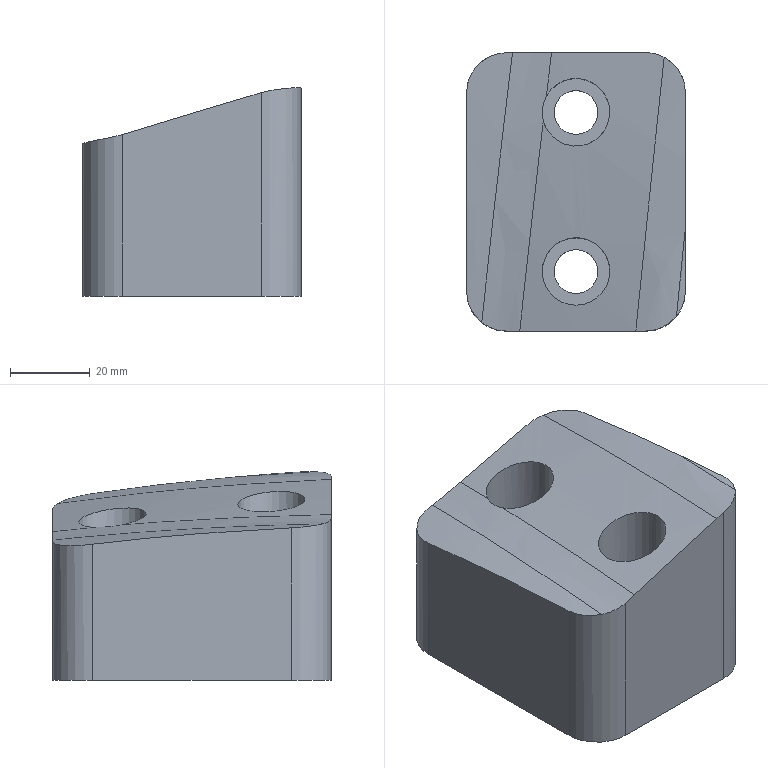Part | NX | features solid 2 | 1 solid | 20 faces | box 55 x 70 x 52.401 mm | volume 147496 mm3 | cylinder 8 | plane 7 | spline 5 | commonest cylinder face diameters 20 x4 11 x2 17 x2
STEP:
#1=CARTESIAN_POINT('',(-250.,310.,23.05));
#2=VERTEX_POINT('',#1);
#3=CARTESIAN_POINT('',(-273.631,310.,17.313));
#4=VERTEX_POINT('',#3);
#5=CARTESIAN_POINT('',(-250.,310.,23.05));
#6=CARTESIAN_POINT('',(-257.879,310.,21.145));
#7=CARTESIAN_POINT('',(-265.756,310.,19.234));
#8=CARTESIAN_POINT('',(-273.631,310.,17.313));
#9=B_SPLINE_CURVE_WITH_KNOTS('',3,(#5,#6,#7,#8),.UNSPECIFIED.,.F.,.F.,(4,4),(0.005181,0.0295),.UNSPECIFIED.);
#10=EDGE_CURVE('',#2,#4,#9,.T.);
#11=ORIENTED_EDGE('',*,*,#10,.T.);
#12=CARTESIAN_POINT('',(-274.974,299.048,18.446));
#13=VERTEX_POINT('',#12);
#14=CARTESIAN_POINT('',(-273.631,310.,17.313));
#15=CARTESIAN_POINT('',(-274.07,306.431,17.719));
#16=CARTESIAN_POINT('',(-274.514,302.785,18.097));
#17=CARTESIAN_POINT('',(-274.965,299.055,18.448));
#18=B_SPLINE_CURVE_WITH_KNOTS('',3,(#14,#15,#16,#17),.UNSPECIFIED.,.F.,.F.,(4,4),(0.03901,0.4464),.UNSPECIFIED.);
#19=EDGE_CURVE('',#4,#13,#18,.T.);
#20=ORIENTED_EDGE('',*,*,#19,.T.);
#21=CARTESIAN_POINT('',(-275.72,292.836,18.999));
#22=VERTEX_POINT('',#21);
#23=CARTESIAN_POINT('',(-274.963,299.068,18.447));
#24=CARTESIAN_POINT('',(-274.01,300.817,18.471));
#25=CARTESIAN_POINT('',(-270.799,303.603,18.912));
#26=CARTESIAN_POINT('',(-264.634,303.713,20.424));
#27=CARTESIAN_POINT('',(-259.81,300.02,22.155));
#28=CARTESIAN_POINT('',(-258.326,293.943,23.371));
#29=CARTESIAN_POINT('',(-261.238,288.212,23.347));
#30=CARTESIAN_POINT('',(-267.031,285.826,22.093));
#31=CARTESIAN_POINT('',(-272.858,287.562,20.346));
#32=CARTESIAN_POINT('',(-275.205,290.9,19.356));
#33=CARTESIAN_POINT('',(-275.715,292.816,19.003));
#34=B_SPLINE_CURVE_WITH_KNOTS('',3,(#23,#24,#25,#26,#27,#28,#29,#30,#31,#32,#33),.UNSPECIFIED.,.F.,.F.,(4,1,1,1,1,1,1,1,4),(0.001597,0.007571,0.01355,0.01952,0.02549,0.03147,0.03744,0.04341,0.04939),.UNSPECIFIED.);
#35=EDGE_CURVE('',#13,#22,#34,.T.);
#36=ORIENTED_EDGE('',*,*,#35,.T.);
#37=CARTESIAN_POINT('',(-276.835,283.374,19.727));
#38=VERTEX_POINT('',#37);
#39=CARTESIAN_POINT('',(-275.713,292.829,19.002));
#40=CARTESIAN_POINT('',(-276.083,289.735,19.261));
#41=CARTESIAN_POINT('',(-276.457,286.584,19.503));
#42=CARTESIAN_POINT('',(-276.835,283.374,19.727));
#43=B_SPLINE_CURVE_WITH_KNOTS('',3,(#39,#40,#41,#42),.UNSPECIFIED.,.F.,.F.,(4,4),(0.6703,1.),.UNSPECIFIED.);
#44=EDGE_CURVE('',#22,#38,#43,.T.);
#45=ORIENTED_EDGE('',*,*,#44,.T.);
#46=CARTESIAN_POINT('',(-281.649,240.,21.629));
#47=VERTEX_POINT('',#46);
#48=CARTESIAN_POINT('',(-276.835,283.374,19.727));
#49=CARTESIAN_POINT('',(-278.37,270.039,20.667));
#50=CARTESIAN_POINT('',(-279.977,255.669,21.299));
#51=CARTESIAN_POINT('',(-281.671,240.002,21.622));
#52=B_SPLINE_CURVE_WITH_KNOTS('',3,(#48,#49,#50,#51),.UNSPECIFIED.,.F.,.F.,(4,4),(0.,1.502),.UNSPECIFIED.);
#53=EDGE_CURVE('',#38,#47,#52,.T.);
#54=ORIENTED_EDGE('',*,*,#53,.T.);
#55=CARTESIAN_POINT('',(-252.459,240.,30.481));
#56=VERTEX_POINT('',#55);
#57=CARTESIAN_POINT('',(-252.459,240.,30.481));
#58=CARTESIAN_POINT('',(-262.204,240.,27.579));
#59=CARTESIAN_POINT('',(-271.934,240.,24.63));
#60=CARTESIAN_POINT('',(-281.649,240.,21.629));
#61=B_SPLINE_CURVE_WITH_KNOTS('',3,(#57,#58,#59,#60),.UNSPECIFIED.,.F.,.F.,(4,4),(0.1228,0.1533),.UNSPECIFIED.);
#62=EDGE_CURVE('',#47,#56,#61,.F.);
#63=ORIENTED_EDGE('',*,*,#62,.T.);
#64=CARTESIAN_POINT('',(-247.544,288.029,26.924));
#65=VERTEX_POINT('',#64);
#66=CARTESIAN_POINT('',(-252.459,240.,30.481));
#67=CARTESIAN_POINT('',(-250.751,256.963,29.719));
#68=CARTESIAN_POINT('',(-249.117,272.921,28.534));
#69=CARTESIAN_POINT('',(-247.544,288.029,26.924));
#70=B_SPLINE_CURVE_WITH_KNOTS('',3,(#66,#67,#68,#69),.UNSPECIFIED.,.F.,.F.,(4,4),(0.02255,1.),.UNSPECIFIED.);
#71=EDGE_CURVE('',#56,#65,#70,.T.);
#72=ORIENTED_EDGE('',*,*,#71,.T.);
#73=CARTESIAN_POINT('',(-245.332,308.844,24.37));
#74=VERTEX_POINT('',#73);
#75=CARTESIAN_POINT('',(-247.544,288.029,26.924));
#76=CARTESIAN_POINT('',(-246.792,295.151,26.168));
#77=CARTESIAN_POINT('',(-246.054,302.084,25.317));
#78=CARTESIAN_POINT('',(-245.328,308.843,24.371));
#79=B_SPLINE_CURVE_WITH_KNOTS('',3,(#75,#76,#77,#78),.UNSPECIFIED.,.F.,.F.,(4,4),(0.,0.5687),.UNSPECIFIED.);
#80=EDGE_CURVE('',#65,#74,#79,.T.);
#81=ORIENTED_EDGE('',*,*,#80,.T.);
#82=CARTESIAN_POINT('',(-250.,310.,23.05));
#83=CARTESIAN_POINT('',(-248.355,310.,23.447));
#84=CARTESIAN_POINT('',(-246.764,309.6,23.898));
#85=CARTESIAN_POINT('',(-245.328,308.841,24.371));
#86=B_SPLINE_CURVE_WITH_KNOTS('',3,(#82,#83,#84,#85),.UNSPECIFIED.,.F.,.F.,(4,4),(0.,0.005003),.UNSPECIFIED.);
#87=EDGE_CURVE('',#2,#74,#86,.T.);
#88=ORIENTED_EDGE('',*,*,#87,.F.);
#89=EDGE_LOOP('',(#11,#20,#36,#45,#54,#63,#72,#81,#88));
#90=FACE_BOUND('',#89,.T.);
#91=CARTESIAN_POINT('',(-259.,255.,27.364));
#92=VERTEX_POINT('',#91);
#93=CARTESIAN_POINT('',(-260.918,261.697,26.225));
#94=CARTESIAN_POINT('',(-258.03,255.03,27.651));
#95=CARTESIAN_POINT('',(-260.962,248.181,27.355));
#96=CARTESIAN_POINT('',(-267.618,245.634,25.552));
#97=CARTESIAN_POINT('',(-274.069,248.287,23.435));
#98=CARTESIAN_POINT('',(-276.967,254.958,22.125));
#99=CARTESIAN_POINT('',(-274.061,261.802,22.466));
#100=CARTESIAN_POINT('',(-267.366,264.374,24.157));
#101=CARTESIAN_POINT('',(-260.918,261.697,26.225));
#102=CARTESIAN_POINT('',(-258.03,255.03,27.651));
#103=CARTESIAN_POINT('',(-260.962,248.181,27.355));
#104=B_SPLINE_CURVE_WITH_KNOTS('',3,(#93,#94,#95,#96,#97,#98,#99,#100,#101,#102,#103),.UNSPECIFIED.,.T.,.F.,(1,1,1,1,1,1,1,1,1,1,1,1,1,1,1),(-0.02039,-0.01359,-0.006795,0.,0.006795,0.01359,0.02039,0.02718,0.03398,0.04077,0.04757,0.05436,0.06116,0.06795,0.07475),.UNSPECIFIED.);
#105=EDGE_CURVE('',#92,#92,#104,.T.);
#106=ORIENTED_EDGE('',*,*,#105,.T.);
#107=EDGE_LOOP('',(#106));
#108=FACE_BOUND('',#107,.T.);
#109=CARTESIAN_POINT('',(-281.891,239.57,21.577));
#110=CARTESIAN_POINT('',(-280.657,251.406,21.326));
#111=CARTESIAN_POINT('',(-279.46,262.664,20.939));
#112=CARTESIAN_POINT('',(-278.301,273.385,20.416));
#113=CARTESIAN_POINT('',(-277.175,283.609,19.758));
#114=CARTESIAN_POINT('',(-276.082,293.377,18.967));
#115=CARTESIAN_POINT('',(-275.019,302.722,18.042));
#116=CARTESIAN_POINT('',(-273.985,311.672,16.985));
#117=CARTESIAN_POINT('',(-253.323,229.701,30.94));
#118=CARTESIAN_POINT('',(-252.047,242.381,30.507));
#119=CARTESIAN_POINT('',(-250.803,254.633,29.899));
#120=CARTESIAN_POINT('',(-249.59,266.479,29.116));
#121=CARTESIAN_POINT('',(-248.404,277.941,28.156));
#122=CARTESIAN_POINT('',(-247.243,289.043,27.02));
#123=CARTESIAN_POINT('',(-246.107,299.802,25.708));
#124=CARTESIAN_POINT('',(-244.993,310.238,24.219));
#125=B_SPLINE_SURFACE_WITH_KNOTS('',1,7,((#109,#110,#111,#112,#113,#114,#115,#116),(#117,#118,#119,#120,#121,#122,#123,#124)),.RULED_SURF.,.F.,.F.,.F.,(2,2),(8,8),(0.0009795,0.9981),(0.7451,0.9196),.PIECEWISE_BEZIER_KNOTS.);
#126=ADVANCED_FACE('',(#90,#108),#125,.T.);
#127=CARTESIAN_POINT('',(-262.,255.,-20.));
#128=VERTEX_POINT('',#127);
#129=CARTESIAN_POINT('',(-267.5,255.,-20.));
#130=DIRECTION('',(0.,0.,1.));
#131=DIRECTION('',(1.,0.,0.));
#132=AXIS2_PLACEMENT_3D('',#129,#130,#131);
#133=CIRCLE('',#132,5.5);
#134=EDGE_CURVE('',#128,#128,#133,.F.);
#135=ORIENTED_EDGE('',*,*,#134,.T.);
#136=EDGE_LOOP('',(#135));
#137=FACE_BOUND('',#136,.T.);
#138=CARTESIAN_POINT('',(-273.,255.,0.));
#139=VERTEX_POINT('',#138);
#140=CARTESIAN_POINT('',(-267.5,255.,0.));
#141=DIRECTION('',(0.,0.,-1.));
#142=DIRECTION('',(-1.,0.,0.));
#143=AXIS2_PLACEMENT_3D('',#140,#141,#142);
#144=CIRCLE('',#143,5.5);
#145=EDGE_CURVE('',#139,#139,#144,.F.);
#146=ORIENTED_EDGE('',*,*,#145,.T.);
#147=EDGE_LOOP('',(#146));
#148=FACE_BOUND('',#147,.T.);
#149=CARTESIAN_POINT('',(-267.5,255.,-20.));
#150=DIRECTION('',(0.,0.,1.));
#151=DIRECTION('',(-1.,0.,0.));
#152=AXIS2_PLACEMENT_3D('',#149,#150,#151);
#153=CYLINDRICAL_SURFACE('',#152,5.5);
#154=ADVANCED_FACE('',(#137,#148),#153,.F.);
#155=CARTESIAN_POINT('',(-285.,240.,20.642));
#156=VERTEX_POINT('',#155);
#157=CARTESIAN_POINT('',(-281.649,240.,21.629));
#158=CARTESIAN_POINT('',(-282.762,240.,21.285));
#159=CARTESIAN_POINT('',(-283.875,240.,20.944));
#160=CARTESIAN_POINT('',(-285.,240.,20.642));
#161=B_SPLINE_CURVE_WITH_KNOTS('',3,(#157,#158,#159,#160),.UNSPECIFIED.,.F.,.F.,(4,4),(0.04027,0.04376),.UNSPECIFIED.);
#162=EDGE_CURVE('',#47,#156,#161,.T.);
#163=ORIENTED_EDGE('',*,*,#162,.F.);
#164=ORIENTED_EDGE('',*,*,#53,.F.);
#165=ORIENTED_EDGE('',*,*,#44,.F.);
#166=CARTESIAN_POINT('',(-274.978,299.042,18.446));
#167=CARTESIAN_POINT('',(-276.005,297.141,18.422));
#168=CARTESIAN_POINT('',(-276.261,294.899,18.62));
#169=CARTESIAN_POINT('',(-275.722,292.842,18.998));
#170=B_SPLINE_CURVE_WITH_KNOTS('',3,(#166,#167,#168,#169),.UNSPECIFIED.,.F.,.F.,(4,4),(0.,0.006389),.UNSPECIFIED.);
#171=EDGE_CURVE('',#13,#22,#170,.T.);
#172=ORIENTED_EDGE('',*,*,#171,.F.);
#173=ORIENTED_EDGE('',*,*,#19,.F.);
#174=CARTESIAN_POINT('',(-283.452,310.,15.17));
#175=VERTEX_POINT('',#174);
#176=CARTESIAN_POINT('',(-283.446,310.,15.171));
#177=CARTESIAN_POINT('',(-280.158,310.,15.803));
#178=CARTESIAN_POINT('',(-276.886,310.,16.519));
#179=CARTESIAN_POINT('',(-273.632,310.,17.313));
#180=B_SPLINE_CURVE_WITH_KNOTS('',3,(#176,#177,#178,#179),.UNSPECIFIED.,.F.,.F.,(4,4),(0.,0.01005),.UNSPECIFIED.);
#181=EDGE_CURVE('',#175,#4,#180,.T.);
#182=ORIENTED_EDGE('',*,*,#181,.F.);
#183=CARTESIAN_POINT('',(-284.194,303.925,15.81));
#184=VERTEX_POINT('',#183);
#185=CARTESIAN_POINT('',(-284.194,303.925,15.81));
#186=CARTESIAN_POINT('',(-283.946,305.955,15.607));
#187=CARTESIAN_POINT('',(-283.697,307.981,15.394));
#188=CARTESIAN_POINT('',(-283.446,310.,15.171));
#189=B_SPLINE_CURVE_WITH_KNOTS('',3,(#185,#186,#187,#188),.UNSPECIFIED.,.F.,.F.,(4,4),(0.,0.2974),.UNSPECIFIED.);
#190=EDGE_CURVE('',#184,#175,#189,.T.);
#191=ORIENTED_EDGE('',*,*,#190,.F.);
#192=CARTESIAN_POINT('',(-287.838,272.864,18.153));
#193=VERTEX_POINT('',#192);
#194=CARTESIAN_POINT('',(-287.838,272.864,18.153));
#195=CARTESIAN_POINT('',(-286.663,283.265,17.593));
#196=CARTESIAN_POINT('',(-285.448,293.654,16.834));
#197=CARTESIAN_POINT('',(-284.194,303.925,15.81));
#198=B_SPLINE_CURVE_WITH_KNOTS('',3,(#194,#195,#196,#197),.UNSPECIFIED.,.F.,.F.,(4,4),(0.,1.),.UNSPECIFIED.);
#199=EDGE_CURVE('',#193,#184,#198,.T.);
#200=ORIENTED_EDGE('',*,*,#199,.F.);
#201=CARTESIAN_POINT('',(-291.202,242.155,19.282));
#202=VERTEX_POINT('',#201);
#203=CARTESIAN_POINT('',(-291.201,242.155,19.282));
#204=CARTESIAN_POINT('',(-290.112,252.398,19.062));
#205=CARTESIAN_POINT('',(-288.994,262.64,18.704));
#206=CARTESIAN_POINT('',(-287.838,272.864,18.153));
#207=B_SPLINE_CURVE_WITH_KNOTS('',3,(#203,#204,#205,#206),.UNSPECIFIED.,.F.,.F.,(4,4),(0.3155,1.),.UNSPECIFIED.);
#208=EDGE_CURVE('',#202,#193,#207,.T.);
#209=ORIENTED_EDGE('',*,*,#208,.F.);
#210=CARTESIAN_POINT('',(-285.,240.,20.642));
#211=CARTESIAN_POINT('',(-287.213,240.,20.048));
#212=CARTESIAN_POINT('',(-289.424,240.75,19.63));
#213=CARTESIAN_POINT('',(-291.201,242.155,19.282));
#214=B_SPLINE_CURVE_WITH_KNOTS('',3,(#210,#211,#212,#213),.UNSPECIFIED.,.F.,.F.,(4,4),(0.,0.006825),.UNSPECIFIED.);
#215=EDGE_CURVE('',#156,#202,#214,.T.);
#216=ORIENTED_EDGE('',*,*,#215,.F.);
#217=EDGE_LOOP('',(#163,#164,#165,#172,#173,#182,#191,#200,#209,#216));
#218=FACE_BOUND('',#217,.T.);
#219=CARTESIAN_POINT('',(-273.447,311.482,17.143));
#220=CARTESIAN_POINT('',(-275.416,311.35,16.685));
#221=CARTESIAN_POINT('',(-277.386,311.212,16.227));
#222=CARTESIAN_POINT('',(-279.368,311.041,15.81));
#223=CARTESIAN_POINT('',(-281.382,310.73,15.469));
#224=CARTESIAN_POINT('',(-283.395,310.411,15.125));
#225=CARTESIAN_POINT('',(-274.718,301.322,18.322));
#226=CARTESIAN_POINT('',(-276.678,301.229,17.838));
#227=CARTESIAN_POINT('',(-278.637,301.133,17.353));
#228=CARTESIAN_POINT('',(-280.612,301.008,16.923));
#229=CARTESIAN_POINT('',(-282.619,300.761,16.578));
#230=CARTESIAN_POINT('',(-284.626,300.508,16.229));
#231=CARTESIAN_POINT('',(-275.964,291.031,19.288));
#232=CARTESIAN_POINT('',(-277.914,290.978,18.779));
#233=CARTESIAN_POINT('',(-279.864,290.923,18.269));
#234=CARTESIAN_POINT('',(-281.832,290.845,17.829));
#235=CARTESIAN_POINT('',(-283.832,290.662,17.483));
#236=CARTESIAN_POINT('',(-285.832,290.475,17.132));
#237=CARTESIAN_POINT('',(-277.176,280.694,20.056));
#238=CARTESIAN_POINT('',(-279.116,280.681,19.525));
#239=CARTESIAN_POINT('',(-281.057,280.666,18.992));
#240=CARTESIAN_POINT('',(-283.018,280.634,18.543));
#241=CARTESIAN_POINT('',(-285.013,280.515,18.198));
#242=CARTESIAN_POINT('',(-287.007,280.393,17.849));
#243=CARTESIAN_POINT('',(-278.354,270.341,20.656));
#244=CARTESIAN_POINT('',(-280.286,270.369,20.104));
#245=CARTESIAN_POINT('',(-282.218,270.394,19.551));
#246=CARTESIAN_POINT('',(-284.174,270.408,19.095));
#247=CARTESIAN_POINT('',(-286.163,270.352,18.753));
#248=CARTESIAN_POINT('',(-288.152,270.294,18.408));
#249=CARTESIAN_POINT('',(-279.504,259.983,21.108));
#250=CARTESIAN_POINT('',(-281.427,260.05,20.538));
#251=CARTESIAN_POINT('',(-283.35,260.117,19.967));
#252=CARTESIAN_POINT('',(-285.301,260.175,19.506));
#253=CARTESIAN_POINT('',(-287.285,260.183,19.169));
#254=CARTESIAN_POINT('',(-289.269,260.188,18.828));
#255=CARTESIAN_POINT('',(-280.628,249.62,21.432));
#256=CARTESIAN_POINT('',(-282.543,249.729,20.847));
#257=CARTESIAN_POINT('',(-284.458,249.836,20.261));
#258=CARTESIAN_POINT('',(-286.403,249.94,19.795));
#259=CARTESIAN_POINT('',(-288.383,250.01,19.465));
#260=CARTESIAN_POINT('',(-290.362,250.079,19.13));
#261=CARTESIAN_POINT('',(-281.728,239.254,21.645));
#262=CARTESIAN_POINT('',(-283.636,239.404,21.046));
#263=CARTESIAN_POINT('',(-285.544,239.553,20.447));
#264=CARTESIAN_POINT('',(-287.484,239.702,19.979));
#265=CARTESIAN_POINT('',(-289.459,239.835,19.655));
#266=CARTESIAN_POINT('',(-291.434,239.967,19.327));
#267=B_SPLINE_SURFACE_WITH_KNOTS('',7,5,((#219,#220,#221,#222,#223,#224),(#225,#226,#227,#228,#229,#230),(#231,#232,#233,#234,#235,#236),(#237,#238,#239,#240,#241,#242),(#243,#244,#245,#246,#247,#248),(#249,#250,#251,#252,#253,#254),(#255,#256,#257,#258,#259,#260),(#261,#262,#263,#264,#265,#266)),.UNSPECIFIED.,.F.,.F.,.F.,(8,8),(6,6),(0.253,0.8919),(0.,1.),.PIECEWISE_BEZIER_KNOTS.);
#268=ADVANCED_FACE('',(#218),#267,.F.);
#269=CARTESIAN_POINT('',(-262.,295.,-20.));
#270=VERTEX_POINT('',#269);
#271=CARTESIAN_POINT('',(-267.5,295.,-20.));
#272=DIRECTION('',(0.,0.,1.));
#273=DIRECTION('',(1.,0.,0.));
#274=AXIS2_PLACEMENT_3D('',#271,#272,#273);
#275=CIRCLE('',#274,5.5);
#276=EDGE_CURVE('',#270,#270,#275,.F.);
#277=ORIENTED_EDGE('',*,*,#276,.T.);
#278=EDGE_LOOP('',(#277));
#279=FACE_BOUND('',#278,.T.);
#280=CARTESIAN_POINT('',(-273.,295.,0.));
#281=VERTEX_POINT('',#280);
#282=CARTESIAN_POINT('',(-267.5,295.,0.));
#283=DIRECTION('',(0.,0.,-1.));
#284=DIRECTION('',(-1.,0.,0.));
#285=AXIS2_PLACEMENT_3D('',#282,#283,#284);
#286=CIRCLE('',#285,5.5);
#287=EDGE_CURVE('',#281,#281,#286,.F.);
#288=ORIENTED_EDGE('',*,*,#287,.T.);
#289=EDGE_LOOP('',(#288));
#290=FACE_BOUND('',#289,.T.);
#291=CARTESIAN_POINT('',(-267.5,295.,-20.));
#292=DIRECTION('',(0.,0.,1.));
#293=DIRECTION('',(-1.,0.,0.));
#294=AXIS2_PLACEMENT_3D('',#291,#292,#293);
#295=CYLINDRICAL_SURFACE('',#294,5.5);
#296=ADVANCED_FACE('',(#279,#290),#295,.F.);
#297=CARTESIAN_POINT('',(-285.,240.,-20.));
#298=VERTEX_POINT('',#297);
#299=CARTESIAN_POINT('',(-250.,240.,-20.));
#300=VERTEX_POINT('',#299);
#301=CARTESIAN_POINT('',(-295.,240.,-20.));
#302=DIRECTION('',(-1.,0.,0.));
#303=VECTOR('',#302,1000.);
#304=LINE('',#301,#303);
#305=EDGE_CURVE('',#298,#300,#304,.F.);
#306=ORIENTED_EDGE('',*,*,#305,.T.);
#307=CARTESIAN_POINT('',(-250.,240.,31.188));
#308=VERTEX_POINT('',#307);
#309=CARTESIAN_POINT('',(-250.,240.,-10.));
#310=DIRECTION('',(0.,0.,-1.));
#311=VECTOR('',#310,1000.);
#312=LINE('',#309,#311);
#313=EDGE_CURVE('',#308,#300,#312,.T.);
#314=ORIENTED_EDGE('',*,*,#313,.F.);
#315=CARTESIAN_POINT('',(-250.,240.,31.188));
#316=CARTESIAN_POINT('',(-250.824,240.,30.967));
#317=CARTESIAN_POINT('',(-251.642,240.,30.724));
#318=CARTESIAN_POINT('',(-252.459,240.,30.481));
#319=B_SPLINE_CURVE_WITH_KNOTS('',3,(#315,#316,#317,#318),.UNSPECIFIED.,.F.,.F.,(4,4),(0.04781,0.05037),.UNSPECIFIED.);
#320=EDGE_CURVE('',#308,#56,#319,.T.);
#321=ORIENTED_EDGE('',*,*,#320,.T.);
#322=ORIENTED_EDGE('',*,*,#62,.F.);
#323=ORIENTED_EDGE('',*,*,#162,.T.);
#324=CARTESIAN_POINT('',(-285.,240.,-10.));
#325=DIRECTION('',(0.,0.,1.));
#326=VECTOR('',#325,1000.);
#327=LINE('',#324,#326);
#328=EDGE_CURVE('',#298,#156,#327,.T.);
#329=ORIENTED_EDGE('',*,*,#328,.F.);
#330=EDGE_LOOP('',(#306,#314,#321,#322,#323,#329));
#331=FACE_BOUND('',#330,.T.);
#332=CARTESIAN_POINT('',(-295.,240.,-10.));
#333=DIRECTION('',(0.,-1.,0.));
#334=DIRECTION('',(1.,0.,0.));
#335=AXIS2_PLACEMENT_3D('',#332,#333,#334);
#336=PLANE('',#335);
#337=ADVANCED_FACE('',(#331),#336,.T.);
#338=CARTESIAN_POINT('',(-240.,250.,-20.));
#339=VERTEX_POINT('',#338);
#340=CARTESIAN_POINT('',(-240.,300.,-20.));
#341=VERTEX_POINT('',#340);
#342=CARTESIAN_POINT('',(-240.,260.,-20.));
#343=DIRECTION('',(0.,-1.,0.));
#344=VECTOR('',#343,1000.);
#345=LINE('',#342,#344);
#346=EDGE_CURVE('',#339,#341,#345,.F.);
#347=ORIENTED_EDGE('',*,*,#346,.T.);
#348=CARTESIAN_POINT('',(-240.,300.,26.917));
#349=VERTEX_POINT('',#348);
#350=CARTESIAN_POINT('',(-240.,300.,-10.));
#351=DIRECTION('',(0.,0.,1.));
#352=VECTOR('',#351,1000.);
#353=LINE('',#350,#352);
#354=EDGE_CURVE('',#349,#341,#353,.F.);
#355=ORIENTED_EDGE('',*,*,#354,.F.);
#356=CARTESIAN_POINT('',(-240.,265.918,30.94));
#357=VERTEX_POINT('',#356);
#358=CARTESIAN_POINT('',(-240.,300.,26.917));
#359=CARTESIAN_POINT('',(-240.,288.681,28.578));
#360=CARTESIAN_POINT('',(-240.,277.313,29.896));
#361=CARTESIAN_POINT('',(-240.,265.92,30.94));
#362=B_SPLINE_CURVE_WITH_KNOTS('',3,(#358,#359,#360,#361),.UNSPECIFIED.,.F.,.F.,(4,4),(0.01012,0.04444),.UNSPECIFIED.);
#363=EDGE_CURVE('',#349,#357,#362,.T.);
#364=ORIENTED_EDGE('',*,*,#363,.T.);
#365=CARTESIAN_POINT('',(-240.,250.,32.23));
#366=VERTEX_POINT('',#365);
#367=CARTESIAN_POINT('',(-240.,265.918,30.94));
#368=CARTESIAN_POINT('',(-240.,260.615,31.426));
#369=CARTESIAN_POINT('',(-240.,255.306,31.855));
#370=CARTESIAN_POINT('',(-240.,250.,32.23));
#371=B_SPLINE_CURVE_WITH_KNOTS('',3,(#367,#368,#369,#370),.UNSPECIFIED.,.F.,.F.,(4,4),(0.02526,0.04123),.UNSPECIFIED.);
#372=EDGE_CURVE('',#357,#366,#371,.T.);
#373=ORIENTED_EDGE('',*,*,#372,.T.);
#374=CARTESIAN_POINT('',(-240.,250.,-10.));
#375=DIRECTION('',(0.,0.,-1.));
#376=VECTOR('',#375,1000.);
#377=LINE('',#374,#376);
#378=EDGE_CURVE('',#339,#366,#377,.F.);
#379=ORIENTED_EDGE('',*,*,#378,.F.);
#380=EDGE_LOOP('',(#347,#355,#364,#373,#379));
#381=FACE_BOUND('',#380,.T.);
#382=CARTESIAN_POINT('',(-240.,260.,-10.));
#383=DIRECTION('',(1.,0.,0.));
#384=DIRECTION('',(0.,1.,0.));
#385=AXIS2_PLACEMENT_3D('',#382,#383,#384);
#386=PLANE('',#385);
#387=ADVANCED_FACE('',(#381),#386,.T.);
#388=CARTESIAN_POINT('',(-285.,310.,14.871));
#389=VERTEX_POINT('',#388);
#390=CARTESIAN_POINT('',(-285.,310.,14.871));
#391=CARTESIAN_POINT('',(-284.485,310.,14.971));
#392=CARTESIAN_POINT('',(-283.969,310.,15.07));
#393=CARTESIAN_POINT('',(-283.454,310.,15.169));
#394=B_SPLINE_CURVE_WITH_KNOTS('',3,(#390,#391,#392,#393),.UNSPECIFIED.,.F.,.F.,(4,4),(0.0102,0.01177),.UNSPECIFIED.);
#395=EDGE_CURVE('',#389,#175,#394,.T.);
#396=ORIENTED_EDGE('',*,*,#395,.T.);
#397=ORIENTED_EDGE('',*,*,#181,.T.);
#398=ORIENTED_EDGE('',*,*,#10,.F.);
#399=CARTESIAN_POINT('',(-250.,310.,-20.));
#400=VERTEX_POINT('',#399);
#401=CARTESIAN_POINT('',(-250.,310.,-10.));
#402=DIRECTION('',(0.,0.,-1.));
#403=VECTOR('',#402,1000.);
#404=LINE('',#401,#403);
#405=EDGE_CURVE('',#400,#2,#404,.F.);
#406=ORIENTED_EDGE('',*,*,#405,.F.);
#407=CARTESIAN_POINT('',(-285.,310.,-20.));
#408=VERTEX_POINT('',#407);
#409=CARTESIAN_POINT('',(-295.,310.,-20.));
#410=DIRECTION('',(1.,0.,0.));
#411=VECTOR('',#410,1000.);
#412=LINE('',#409,#411);
#413=EDGE_CURVE('',#408,#400,#412,.T.);
#414=ORIENTED_EDGE('',*,*,#413,.F.);
#415=CARTESIAN_POINT('',(-285.,310.,-10.));
#416=DIRECTION('',(0.,0.,1.));
#417=VECTOR('',#416,1000.);
#418=LINE('',#415,#417);
#419=EDGE_CURVE('',#389,#408,#418,.F.);
#420=ORIENTED_EDGE('',*,*,#419,.F.);
#421=EDGE_LOOP('',(#396,#397,#398,#406,#414,#420));
#422=FACE_BOUND('',#421,.T.);
#423=CARTESIAN_POINT('',(-295.,310.,-10.));
#424=DIRECTION('',(0.,-1.,0.));
#425=DIRECTION('',(1.,0.,0.));
#426=AXIS2_PLACEMENT_3D('',#423,#424,#425);
#427=PLANE('',#426);
#428=ADVANCED_FACE('',(#422),#427,.F.);
#429=CARTESIAN_POINT('',(-295.,250.,18.299));
#430=VERTEX_POINT('',#429);
#431=CARTESIAN_POINT('',(-295.,300.,14.192));
#432=VERTEX_POINT('',#431);
#433=CARTESIAN_POINT('',(-295.,250.,18.299));
#434=CARTESIAN_POINT('',(-295.,266.7,17.48));
#435=CARTESIAN_POINT('',(-295.,283.395,16.213));
#436=CARTESIAN_POINT('',(-295.,300.,14.192));
#437=B_SPLINE_CURVE_WITH_KNOTS('',3,(#433,#434,#435,#436),.UNSPECIFIED.,.F.,.F.,(4,4),(-0.01001,0.04016),.UNSPECIFIED.);
#438=EDGE_CURVE('',#430,#432,#437,.T.);
#439=ORIENTED_EDGE('',*,*,#438,.T.);
#440=CARTESIAN_POINT('',(-295.,300.,-20.));
#441=VERTEX_POINT('',#440);
#442=CARTESIAN_POINT('',(-295.,300.,-10.));
#443=DIRECTION('',(0.,0.,1.));
#444=VECTOR('',#443,1000.);
#445=LINE('',#442,#444);
#446=EDGE_CURVE('',#441,#432,#445,.T.);
#447=ORIENTED_EDGE('',*,*,#446,.F.);
#448=CARTESIAN_POINT('',(-295.,250.,-20.));
#449=VERTEX_POINT('',#448);
#450=CARTESIAN_POINT('',(-295.,260.,-20.));
#451=DIRECTION('',(0.,1.,0.));
#452=VECTOR('',#451,1000.);
#453=LINE('',#450,#452);
#454=EDGE_CURVE('',#449,#441,#453,.T.);
#455=ORIENTED_EDGE('',*,*,#454,.F.);
#456=CARTESIAN_POINT('',(-295.,250.,-10.));
#457=DIRECTION('',(0.,0.,-1.));
#458=VECTOR('',#457,1000.);
#459=LINE('',#456,#458);
#460=EDGE_CURVE('',#430,#449,#459,.T.);
#461=ORIENTED_EDGE('',*,*,#460,.F.);
#462=EDGE_LOOP('',(#439,#447,#455,#461));
#463=FACE_BOUND('',#462,.T.);
#464=CARTESIAN_POINT('',(-295.,260.,-10.));
#465=DIRECTION('',(1.,0.,0.));
#466=DIRECTION('',(0.,1.,0.));
#467=AXIS2_PLACEMENT_3D('',#464,#465,#466);
#468=PLANE('',#467);
#469=ADVANCED_FACE('',(#463),#468,.F.);
#470=ORIENTED_EDGE('',*,*,#134,.F.);
#471=EDGE_LOOP('',(#470));
#472=FACE_BOUND('',#471,.T.);
#473=ORIENTED_EDGE('',*,*,#276,.F.);
#474=EDGE_LOOP('',(#473));
#475=FACE_BOUND('',#474,.T.);
#476=ORIENTED_EDGE('',*,*,#454,.T.);
#477=CARTESIAN_POINT('',(-285.,300.,-20.));
#478=DIRECTION('',(0.,0.,1.));
#479=DIRECTION('',(1.,0.,0.));
#480=AXIS2_PLACEMENT_3D('',#477,#478,#479);
#481=CIRCLE('',#480,10.);
#482=EDGE_CURVE('',#408,#441,#481,.T.);
#483=ORIENTED_EDGE('',*,*,#482,.F.);
#484=ORIENTED_EDGE('',*,*,#413,.T.);
#485=CARTESIAN_POINT('',(-250.,300.,-20.));
#486=DIRECTION('',(0.,0.,1.));
#487=DIRECTION('',(1.,0.,0.));
#488=AXIS2_PLACEMENT_3D('',#485,#486,#487);
#489=CIRCLE('',#488,10.);
#490=EDGE_CURVE('',#341,#400,#489,.T.);
#491=ORIENTED_EDGE('',*,*,#490,.F.);
#492=ORIENTED_EDGE('',*,*,#346,.F.);
#493=CARTESIAN_POINT('',(-250.,250.,-20.));
#494=DIRECTION('',(0.,0.,1.));
#495=DIRECTION('',(1.,0.,0.));
#496=AXIS2_PLACEMENT_3D('',#493,#494,#495);
#497=CIRCLE('',#496,10.);
#498=EDGE_CURVE('',#300,#339,#497,.T.);
#499=ORIENTED_EDGE('',*,*,#498,.F.);
#500=ORIENTED_EDGE('',*,*,#305,.F.);
#501=CARTESIAN_POINT('',(-285.,250.,-20.));
#502=DIRECTION('',(0.,0.,1.));
#503=DIRECTION('',(1.,0.,0.));
#504=AXIS2_PLACEMENT_3D('',#501,#502,#503);
#505=CIRCLE('',#504,10.);
#506=EDGE_CURVE('',#449,#298,#505,.T.);
#507=ORIENTED_EDGE('',*,*,#506,.F.);
#508=EDGE_LOOP('',(#476,#483,#484,#491,#492,#499,#500,#507));
#509=FACE_BOUND('',#508,.T.);
#510=CARTESIAN_POINT('',(-295.,260.,-20.));
#511=DIRECTION('',(0.,0.,-1.));
#512=DIRECTION('',(1.,0.,0.));
#513=AXIS2_PLACEMENT_3D('',#510,#511,#512);
#514=PLANE('',#513);
#515=ADVANCED_FACE('',(#472,#475,#509),#514,.T.);
#516=ORIENTED_EDGE('',*,*,#372,.F.);
#517=CARTESIAN_POINT('',(-240.092,265.028,31.009));
#518=VERTEX_POINT('',#517);
#519=CARTESIAN_POINT('',(-240.092,265.028,31.009));
#520=CARTESIAN_POINT('',(-240.061,265.324,30.986));
#521=CARTESIAN_POINT('',(-240.03,265.62,30.963));
#522=CARTESIAN_POINT('',(-240.,265.916,30.94));
#523=B_SPLINE_CURVE_WITH_KNOTS('',3,(#519,#520,#521,#522),.UNSPECIFIED.,.F.,.F.,(4,4),(0.,0.01771),.UNSPECIFIED.);
#524=EDGE_CURVE('',#518,#357,#523,.T.);
#525=ORIENTED_EDGE('',*,*,#524,.F.);
#526=CARTESIAN_POINT('',(-242.264,243.664,32.368));
#527=VERTEX_POINT('',#526);
#528=CARTESIAN_POINT('',(-242.262,243.664,32.368));
#529=CARTESIAN_POINT('',(-241.526,250.954,31.996));
#530=CARTESIAN_POINT('',(-240.803,258.071,31.543));
#531=CARTESIAN_POINT('',(-240.092,265.028,31.009));
#532=B_SPLINE_CURVE_WITH_KNOTS('',3,(#528,#529,#530,#531),.UNSPECIFIED.,.F.,.F.,(4,4),(0.6908,1.),.UNSPECIFIED.);
#533=EDGE_CURVE('',#527,#518,#532,.T.);
#534=ORIENTED_EDGE('',*,*,#533,.F.);
#535=CARTESIAN_POINT('',(-240.,250.,32.23));
#536=CARTESIAN_POINT('',(-240.,247.695,32.394));
#537=CARTESIAN_POINT('',(-240.799,245.454,32.44));
#538=CARTESIAN_POINT('',(-242.262,243.666,32.368));
#539=B_SPLINE_CURVE_WITH_KNOTS('',3,(#535,#536,#537,#538),.UNSPECIFIED.,.F.,.F.,(4,4),(0.,0.006835),.UNSPECIFIED.);
#540=EDGE_CURVE('',#366,#527,#539,.T.);
#541=ORIENTED_EDGE('',*,*,#540,.F.);
#542=EDGE_LOOP('',(#516,#525,#534,#541));
#543=FACE_BOUND('',#542,.T.);
#544=CARTESIAN_POINT('',(-238.255,266.358,31.133));
#545=CARTESIAN_POINT('',(-238.613,266.294,31.092));
#546=CARTESIAN_POINT('',(-238.97,266.231,31.05));
#547=CARTESIAN_POINT('',(-239.327,266.167,31.008));
#548=CARTESIAN_POINT('',(-239.684,266.103,30.966));
#549=CARTESIAN_POINT('',(-240.041,266.039,30.924));
#550=CARTESIAN_POINT('',(-238.694,261.965,31.477));
#551=CARTESIAN_POINT('',(-239.052,261.902,31.435));
#552=CARTESIAN_POINT('',(-239.409,261.838,31.394));
#553=CARTESIAN_POINT('',(-239.767,261.774,31.352));
#554=CARTESIAN_POINT('',(-240.124,261.71,31.31));
#555=CARTESIAN_POINT('',(-240.482,261.646,31.268));
#556=CARTESIAN_POINT('',(-239.136,257.519,31.794));
#557=CARTESIAN_POINT('',(-239.495,257.455,31.752));
#558=CARTESIAN_POINT('',(-239.853,257.392,31.71));
#559=CARTESIAN_POINT('',(-240.211,257.328,31.669));
#560=CARTESIAN_POINT('',(-240.569,257.264,31.627));
#561=CARTESIAN_POINT('',(-240.927,257.199,31.585));
#562=CARTESIAN_POINT('',(-239.583,253.017,32.083));
#563=CARTESIAN_POINT('',(-239.941,252.954,32.042));
#564=CARTESIAN_POINT('',(-240.3,252.89,32.));
#565=CARTESIAN_POINT('',(-240.659,252.826,31.958));
#566=CARTESIAN_POINT('',(-241.017,252.762,31.917));
#567=CARTESIAN_POINT('',(-241.376,252.698,31.875));
#568=CARTESIAN_POINT('',(-240.033,248.46,32.346));
#569=CARTESIAN_POINT('',(-240.392,248.396,32.304));
#570=CARTESIAN_POINT('',(-240.751,248.332,32.263));
#571=CARTESIAN_POINT('',(-241.111,248.269,32.221));
#572=CARTESIAN_POINT('',(-241.47,248.204,32.179));
#573=CARTESIAN_POINT('',(-241.829,248.14,32.138));
#574=CARTESIAN_POINT('',(-240.487,243.844,32.581));
#575=CARTESIAN_POINT('',(-240.847,243.781,32.54));
#576=CARTESIAN_POINT('',(-241.207,243.717,32.499));
#577=CARTESIAN_POINT('',(-241.567,243.653,32.457));
#578=CARTESIAN_POINT('',(-241.926,243.589,32.415));
#579=CARTESIAN_POINT('',(-242.286,243.525,32.374));
#580=B_SPLINE_SURFACE_WITH_KNOTS('',5,5,((#544,#545,#546,#547,#548,#549),(#550,#551,#552,#553,#554,#555),(#556,#557,#558,#559,#560,#561),(#562,#563,#564,#565,#566,#567),(#568,#569,#570,#571,#572,#573),(#574,#575,#576,#577,#578,#579)),.UNSPECIFIED.,.F.,.F.,.F.,(6,6),(6,6),(0.3894,0.4239),(0.9816,0.9892),.PIECEWISE_BEZIER_KNOTS.);
#581=ADVANCED_FACE('',(#543),#580,.F.);
#582=ORIENTED_EDGE('',*,*,#533,.T.);
#583=ORIENTED_EDGE('',*,*,#524,.T.);
#584=ORIENTED_EDGE('',*,*,#363,.F.);
#585=CARTESIAN_POINT('',(-245.328,308.841,24.371));
#586=CARTESIAN_POINT('',(-242.14,307.157,25.422));
#587=CARTESIAN_POINT('',(-240.,303.719,26.372));
#588=CARTESIAN_POINT('',(-240.,300.,26.917));
#589=B_SPLINE_CURVE_WITH_KNOTS('',3,(#585,#586,#587,#588),.UNSPECIFIED.,.F.,.F.,(4,4),(0.,0.01111),.UNSPECIFIED.);
#590=EDGE_CURVE('',#74,#349,#589,.T.);
#591=ORIENTED_EDGE('',*,*,#590,.F.);
#592=ORIENTED_EDGE('',*,*,#80,.F.);
#593=ORIENTED_EDGE('',*,*,#71,.F.);
#594=ORIENTED_EDGE('',*,*,#320,.F.);
#595=CARTESIAN_POINT('',(-242.262,243.666,32.368));
#596=CARTESIAN_POINT('',(-244.166,241.34,32.274));
#597=CARTESIAN_POINT('',(-247.096,240.,31.968));
#598=CARTESIAN_POINT('',(-250.,240.,31.188));
#599=B_SPLINE_CURVE_WITH_KNOTS('',3,(#595,#596,#597,#598),.UNSPECIFIED.,.F.,.F.,(4,4),(0.,0.008896),.UNSPECIFIED.);
#600=EDGE_CURVE('',#527,#308,#599,.T.);
#601=ORIENTED_EDGE('',*,*,#600,.F.);
#602=EDGE_LOOP('',(#582,#583,#584,#591,#592,#593,#594,#601));
#603=FACE_BOUND('',#602,.T.);
#604=CARTESIAN_POINT('',(-235.268,310.336,26.083));
#605=CARTESIAN_POINT('',(-235.281,310.335,26.082));
#606=CARTESIAN_POINT('',(-235.294,310.334,26.08));
#607=CARTESIAN_POINT('',(-235.306,310.333,26.078));
#608=CARTESIAN_POINT('',(-235.319,310.331,26.077));
#609=CARTESIAN_POINT('',(-235.332,310.33,26.075));
#610=CARTESIAN_POINT('',(-237.339,310.142,25.805));
#611=CARTESIAN_POINT('',(-239.346,309.951,25.532));
#612=CARTESIAN_POINT('',(-241.339,309.739,25.185));
#613=CARTESIAN_POINT('',(-243.316,309.497,24.749));
#614=CARTESIAN_POINT('',(-245.292,309.257,24.31));
#615=CARTESIAN_POINT('',(-236.35,300.321,27.528));
#616=CARTESIAN_POINT('',(-236.363,300.32,27.526));
#617=CARTESIAN_POINT('',(-236.376,300.319,27.524));
#618=CARTESIAN_POINT('',(-236.388,300.318,27.523));
#619=CARTESIAN_POINT('',(-236.401,300.317,27.521));
#620=CARTESIAN_POINT('',(-236.414,300.316,27.519));
#621=CARTESIAN_POINT('',(-238.421,300.138,27.251));
#622=CARTESIAN_POINT('',(-240.428,299.96,26.98));
#623=CARTESIAN_POINT('',(-242.419,299.761,26.623));
#624=CARTESIAN_POINT('',(-244.391,299.532,26.167));
#625=CARTESIAN_POINT('',(-246.363,299.307,25.709));
#626=CARTESIAN_POINT('',(-237.417,290.277,28.777));
#627=CARTESIAN_POINT('',(-237.43,290.276,28.776));
#628=CARTESIAN_POINT('',(-237.442,290.275,28.774));
#629=CARTESIAN_POINT('',(-237.455,290.274,28.772));
#630=CARTESIAN_POINT('',(-237.468,290.273,28.77));
#631=CARTESIAN_POINT('',(-237.48,290.272,28.769));
#632=CARTESIAN_POINT('',(-239.488,290.111,28.502));
#633=CARTESIAN_POINT('',(-241.494,289.951,28.232));
#634=CARTESIAN_POINT('',(-243.482,289.769,27.866));
#635=CARTESIAN_POINT('',(-245.449,289.56,27.389));
#636=CARTESIAN_POINT('',(-247.416,289.354,26.909));
#637=CARTESIAN_POINT('',(-238.47,280.215,29.845));
#638=CARTESIAN_POINT('',(-238.483,280.214,29.843));
#639=CARTESIAN_POINT('',(-238.496,280.213,29.841));
#640=CARTESIAN_POINT('',(-238.508,280.212,29.839));
#641=CARTESIAN_POINT('',(-238.521,280.211,29.838));
#642=CARTESIAN_POINT('',(-238.534,280.21,29.836));
#643=CARTESIAN_POINT('',(-240.54,280.07,29.572));
#644=CARTESIAN_POINT('',(-242.547,279.929,29.304));
#645=CARTESIAN_POINT('',(-244.531,279.768,28.928));
#646=CARTESIAN_POINT('',(-246.493,279.58,28.43));
#647=CARTESIAN_POINT('',(-248.454,279.395,27.93));
#648=CARTESIAN_POINT('',(-239.513,270.134,30.744));
#649=CARTESIAN_POINT('',(-239.525,270.134,30.742));
#650=CARTESIAN_POINT('',(-239.538,270.133,30.74));
#651=CARTESIAN_POINT('',(-239.551,270.132,30.739));
#652=CARTESIAN_POINT('',(-239.563,270.131,30.737));
#653=CARTESIAN_POINT('',(-239.576,270.131,30.735));
#654=CARTESIAN_POINT('',(-241.582,270.011,30.474));
#655=CARTESIAN_POINT('',(-243.588,269.891,30.209));
#656=CARTESIAN_POINT('',(-245.57,269.751,29.824));
#657=CARTESIAN_POINT('',(-247.526,269.586,29.306));
#658=CARTESIAN_POINT('',(-249.481,269.423,28.786));
#659=CARTESIAN_POINT('',(-240.546,260.038,31.488));
#660=CARTESIAN_POINT('',(-240.559,260.038,31.486));
#661=CARTESIAN_POINT('',(-240.571,260.037,31.485));
#662=CARTESIAN_POINT('',(-240.584,260.036,31.483));
#663=CARTESIAN_POINT('',(-240.597,260.036,31.482));
#664=CARTESIAN_POINT('',(-240.609,260.035,31.48));
#665=CARTESIAN_POINT('',(-242.615,259.937,31.222));
#666=CARTESIAN_POINT('',(-244.621,259.837,30.961));
#667=CARTESIAN_POINT('',(-246.6,259.719,30.567));
#668=CARTESIAN_POINT('',(-248.55,259.576,30.031));
#669=CARTESIAN_POINT('',(-250.5,259.437,29.493));
#670=CARTESIAN_POINT('',(-241.571,249.93,32.091));
#671=CARTESIAN_POINT('',(-241.584,249.93,32.089));
#672=CARTESIAN_POINT('',(-241.597,249.929,32.088));
#673=CARTESIAN_POINT('',(-241.61,249.929,32.086));
#674=CARTESIAN_POINT('',(-241.622,249.928,32.084));
#675=CARTESIAN_POINT('',(-241.635,249.928,32.083));
#676=CARTESIAN_POINT('',(-243.641,249.85,31.829));
#677=CARTESIAN_POINT('',(-245.646,249.771,31.571));
#678=CARTESIAN_POINT('',(-247.622,249.674,31.171));
#679=CARTESIAN_POINT('',(-249.567,249.555,30.618));
#680=CARTESIAN_POINT('',(-251.511,249.438,30.062));
#681=CARTESIAN_POINT('',(-242.59,239.815,32.563));
#682=CARTESIAN_POINT('',(-242.603,239.814,32.562));
#683=CARTESIAN_POINT('',(-242.615,239.814,32.56));
#684=CARTESIAN_POINT('',(-242.628,239.814,32.559));
#685=CARTESIAN_POINT('',(-242.641,239.813,32.557));
#686=CARTESIAN_POINT('',(-242.653,239.813,32.556));
#687=CARTESIAN_POINT('',(-244.659,239.755,32.306));
#688=CARTESIAN_POINT('',(-246.664,239.696,32.053));
#689=CARTESIAN_POINT('',(-248.637,239.621,31.647));
#690=CARTESIAN_POINT('',(-250.577,239.526,31.078));
#691=CARTESIAN_POINT('',(-252.516,239.432,30.506));
#692=B_SPLINE_SURFACE_WITH_KNOTS('',7,5,((#604,#605,#606,#607,#608,#609,#610,#611,#612,#613,#614),(#615,#616,#617,#618,#619,#620,#621,#622,#623,#624,#625),(#626,#627,#628,#629,#630,#631,#632,#633,#634,#635,#636),(#637,#638,#639,#640,#641,#642,#643,#644,#645,#646,#647),(#648,#649,#650,#651,#652,#653,#654,#655,#656,#657,#658),(#659,#660,#661,#662,#663,#664,#665,#666,#667,#668,#669),(#670,#671,#672,#673,#674,#675,#676,#677,#678,#679,#680),(#681,#682,#683,#684,#685,#686,#687,#688,#689,#690,#691)),.UNSPECIFIED.,.F.,.F.,.F.,(8,8),(6,5,6),(0.1347,0.4168),(-0.006336,0.,1.),.PIECEWISE_BEZIER_KNOTS.);
#693=ADVANCED_FACE('',(#603),#692,.F.);
#694=ORIENTED_EDGE('',*,*,#208,.T.);
#695=ORIENTED_EDGE('',*,*,#199,.T.);
#696=ORIENTED_EDGE('',*,*,#190,.T.);
#697=ORIENTED_EDGE('',*,*,#395,.F.);
#698=CARTESIAN_POINT('',(-295.,300.,14.192));
#699=CARTESIAN_POINT('',(-295.,302.636,13.872));
#700=CARTESIAN_POINT('',(-292.806,307.857,13.63));
#701=CARTESIAN_POINT('',(-287.606,310.,14.366));
#702=CARTESIAN_POINT('',(-285.,310.,14.871));
#703=B_SPLINE_CURVE_WITH_KNOTS('',3,(#698,#699,#700,#701,#702),.UNSPECIFIED.,.F.,.F.,(4,1,4),(0.,0.007855,0.01571),.UNSPECIFIED.);
#704=EDGE_CURVE('',#432,#389,#703,.T.);
#705=ORIENTED_EDGE('',*,*,#704,.F.);
#706=ORIENTED_EDGE('',*,*,#438,.F.);
#707=CARTESIAN_POINT('',(-291.201,242.155,19.282));
#708=CARTESIAN_POINT('',(-293.567,244.025,18.82));
#709=CARTESIAN_POINT('',(-295.,246.953,18.449));
#710=CARTESIAN_POINT('',(-295.,250.,18.299));
#711=B_SPLINE_CURVE_WITH_KNOTS('',3,(#707,#708,#709,#710),.UNSPECIFIED.,.F.,.F.,(4,4),(0.,0.009022),.UNSPECIFIED.);
#712=EDGE_CURVE('',#202,#430,#711,.T.);
#713=ORIENTED_EDGE('',*,*,#712,.F.);
#714=EDGE_LOOP('',(#694,#695,#696,#697,#705,#706,#713));
#715=FACE_BOUND('',#714,.T.);
#716=CARTESIAN_POINT('',(-283.394,311.05,15.038));
#717=CARTESIAN_POINT('',(-286.034,310.418,14.616));
#718=CARTESIAN_POINT('',(-288.667,309.779,14.188));
#719=CARTESIAN_POINT('',(-291.293,309.132,13.754));
#720=CARTESIAN_POINT('',(-293.91,308.477,13.316));
#721=CARTESIAN_POINT('',(-296.52,307.815,12.872));
#722=CARTESIAN_POINT('',(-283.179,298.778,16.758));
#723=CARTESIAN_POINT('',(-285.817,298.153,16.338));
#724=CARTESIAN_POINT('',(-288.447,297.52,15.913));
#725=CARTESIAN_POINT('',(-291.07,296.88,15.483));
#726=CARTESIAN_POINT('',(-293.685,296.232,15.048));
#727=CARTESIAN_POINT('',(-296.292,295.577,14.607));
#728=CARTESIAN_POINT('',(-282.928,285.978,18.158));
#729=CARTESIAN_POINT('',(-285.562,285.359,17.744));
#730=CARTESIAN_POINT('',(-288.189,284.733,17.324));
#731=CARTESIAN_POINT('',(-290.808,284.099,16.899));
#732=CARTESIAN_POINT('',(-293.42,283.458,16.47));
#733=CARTESIAN_POINT('',(-296.024,282.809,16.035));
#734=CARTESIAN_POINT('',(-282.623,272.601,19.27));
#735=CARTESIAN_POINT('',(-285.253,271.988,18.863));
#736=CARTESIAN_POINT('',(-287.876,271.368,18.451));
#737=CARTESIAN_POINT('',(-290.491,270.741,18.033));
#738=CARTESIAN_POINT('',(-293.099,270.106,17.611));
#739=CARTESIAN_POINT('',(-295.699,269.464,17.183));
#740=CARTESIAN_POINT('',(-282.246,258.598,20.121));
#741=CARTESIAN_POINT('',(-284.871,257.992,19.722));
#742=CARTESIAN_POINT('',(-287.489,257.378,19.318));
#743=CARTESIAN_POINT('',(-290.099,256.758,18.909));
#744=CARTESIAN_POINT('',(-292.702,256.129,18.496));
#745=CARTESIAN_POINT('',(-295.298,255.494,18.077));
#746=CARTESIAN_POINT('',(-281.779,243.921,20.73));
#747=CARTESIAN_POINT('',(-284.398,243.321,20.341));
#748=CARTESIAN_POINT('',(-287.011,242.715,19.947));
#749=CARTESIAN_POINT('',(-289.615,242.1,19.548));
#750=CARTESIAN_POINT('',(-292.213,241.479,19.144));
#751=CARTESIAN_POINT('',(-294.803,240.85,18.736));
#752=B_SPLINE_SURFACE_WITH_KNOTS('',5,5,((#716,#717,#718,#719,#720,#721),(#722,#723,#724,#725,#726,#727),(#728,#729,#730,#731,#732,#733),(#734,#735,#736,#737,#738,#739),(#740,#741,#742,#743,#744,#745),(#746,#747,#748,#749,#750,#751)),.UNSPECIFIED.,.F.,.F.,.F.,(6,6),(6,6),(0.06605,0.221),(0.01502,0.04616),.PIECEWISE_BEZIER_KNOTS.);
#753=ADVANCED_FACE('',(#715),#752,.F.);
#754=CARTESIAN_POINT('',(-276.,295.,0.));
#755=VERTEX_POINT('',#754);
#756=CARTESIAN_POINT('',(-267.5,295.,0.));
#757=DIRECTION('',(0.,0.,-1.));
#758=DIRECTION('',(-1.,0.,0.));
#759=AXIS2_PLACEMENT_3D('',#756,#757,#758);
#760=CIRCLE('',#759,8.5);
#761=EDGE_CURVE('',#755,#755,#760,.T.);
#762=ORIENTED_EDGE('',*,*,#761,.T.);
#763=EDGE_LOOP('',(#762));
#764=FACE_BOUND('',#763,.T.);
#765=ORIENTED_EDGE('',*,*,#35,.F.);
#766=ORIENTED_EDGE('',*,*,#171,.T.);
#767=EDGE_LOOP('',(#765,#766));
#768=FACE_BOUND('',#767,.T.);
#769=CARTESIAN_POINT('',(-267.5,295.,180.));
#770=DIRECTION('',(0.,0.,-1.));
#771=DIRECTION('',(1.,0.,0.));
#772=AXIS2_PLACEMENT_3D('',#769,#770,#771);
#773=CYLINDRICAL_SURFACE('',#772,8.5);
#774=ADVANCED_FACE('',(#764,#768),#773,.F.);
#775=ORIENTED_EDGE('',*,*,#761,.F.);
#776=EDGE_LOOP('',(#775));
#777=FACE_BOUND('',#776,.T.);
#778=ORIENTED_EDGE('',*,*,#287,.F.);
#779=EDGE_LOOP('',(#778));
#780=FACE_BOUND('',#779,.T.);
#781=CARTESIAN_POINT('',(-267.5,295.,0.));
#782=DIRECTION('',(0.,0.,1.));
#783=DIRECTION('',(-1.,0.,0.));
#784=AXIS2_PLACEMENT_3D('',#781,#782,#783);
#785=PLANE('',#784);
#786=ADVANCED_FACE('',(#777,#780),#785,.T.);
#787=CARTESIAN_POINT('',(-276.,255.,0.));
#788=VERTEX_POINT('',#787);
#789=CARTESIAN_POINT('',(-267.5,255.,0.));
#790=DIRECTION('',(0.,0.,-1.));
#791=DIRECTION('',(-1.,0.,0.));
#792=AXIS2_PLACEMENT_3D('',#789,#790,#791);
#793=CIRCLE('',#792,8.5);
#794=EDGE_CURVE('',#788,#788,#793,.T.);
#795=ORIENTED_EDGE('',*,*,#794,.T.);
#796=EDGE_LOOP('',(#795));
#797=FACE_BOUND('',#796,.T.);
#798=ORIENTED_EDGE('',*,*,#105,.F.);
#799=EDGE_LOOP('',(#798));
#800=FACE_BOUND('',#799,.T.);
#801=CARTESIAN_POINT('',(-267.5,255.,180.));
#802=DIRECTION('',(0.,0.,-1.));
#803=DIRECTION('',(1.,0.,0.));
#804=AXIS2_PLACEMENT_3D('',#801,#802,#803);
#805=CYLINDRICAL_SURFACE('',#804,8.5);
#806=ADVANCED_FACE('',(#797,#800),#805,.F.);
#807=ORIENTED_EDGE('',*,*,#794,.F.);
#808=EDGE_LOOP('',(#807));
#809=FACE_BOUND('',#808,.T.);
#810=ORIENTED_EDGE('',*,*,#145,.F.);
#811=EDGE_LOOP('',(#810));
#812=FACE_BOUND('',#811,.T.);
#813=CARTESIAN_POINT('',(-267.5,255.,0.));
#814=DIRECTION('',(0.,0.,1.));
#815=DIRECTION('',(-1.,0.,0.));
#816=AXIS2_PLACEMENT_3D('',#813,#814,#815);
#817=PLANE('',#816);
#818=ADVANCED_FACE('',(#809,#812),#817,.T.);
#819=ORIENTED_EDGE('',*,*,#506,.T.);
#820=ORIENTED_EDGE('',*,*,#328,.T.);
#821=ORIENTED_EDGE('',*,*,#215,.T.);
#822=ORIENTED_EDGE('',*,*,#712,.T.);
#823=ORIENTED_EDGE('',*,*,#460,.T.);
#824=EDGE_LOOP('',(#819,#820,#821,#822,#823));
#825=FACE_BOUND('',#824,.T.);
#826=CARTESIAN_POINT('',(-285.,250.,-10.));
#827=DIRECTION('',(0.,0.,-1.));
#828=DIRECTION('',(1.,0.,0.));
#829=AXIS2_PLACEMENT_3D('',#826,#827,#828);
#830=CYLINDRICAL_SURFACE('',#829,10.);
#831=ADVANCED_FACE('',(#825),#830,.T.);
#832=ORIENTED_EDGE('',*,*,#498,.T.);
#833=ORIENTED_EDGE('',*,*,#378,.T.);
#834=ORIENTED_EDGE('',*,*,#540,.T.);
#835=ORIENTED_EDGE('',*,*,#600,.T.);
#836=ORIENTED_EDGE('',*,*,#313,.T.);
#837=EDGE_LOOP('',(#832,#833,#834,#835,#836));
#838=FACE_BOUND('',#837,.T.);
#839=CARTESIAN_POINT('',(-250.,250.,-10.));
#840=DIRECTION('',(0.,0.,1.));
#841=DIRECTION('',(-1.,0.,0.));
#842=AXIS2_PLACEMENT_3D('',#839,#840,#841);
#843=CYLINDRICAL_SURFACE('',#842,10.);
#844=ADVANCED_FACE('',(#838),#843,.T.);
#845=ORIENTED_EDGE('',*,*,#482,.T.);
#846=ORIENTED_EDGE('',*,*,#446,.T.);
#847=ORIENTED_EDGE('',*,*,#704,.T.);
#848=ORIENTED_EDGE('',*,*,#419,.T.);
#849=EDGE_LOOP('',(#845,#846,#847,#848));
#850=FACE_BOUND('',#849,.T.);
#851=CARTESIAN_POINT('',(-285.,300.,-10.));
#852=DIRECTION('',(0.,0.,1.));
#853=DIRECTION('',(-1.,0.,0.));
#854=AXIS2_PLACEMENT_3D('',#851,#852,#853);
#855=CYLINDRICAL_SURFACE('',#854,10.);
#856=ADVANCED_FACE('',(#850),#855,.T.);
#857=ORIENTED_EDGE('',*,*,#490,.T.);
#858=ORIENTED_EDGE('',*,*,#405,.T.);
#859=ORIENTED_EDGE('',*,*,#87,.T.);
#860=ORIENTED_EDGE('',*,*,#590,.T.);
#861=ORIENTED_EDGE('',*,*,#354,.T.);
#862=EDGE_LOOP('',(#857,#858,#859,#860,#861));
#863=FACE_BOUND('',#862,.T.);
#864=CARTESIAN_POINT('',(-250.,300.,-10.));
#865=DIRECTION('',(0.,0.,-1.));
#866=DIRECTION('',(1.,0.,0.));
#867=AXIS2_PLACEMENT_3D('',#864,#865,#866);
#868=CYLINDRICAL_SURFACE('',#867,10.);
#869=ADVANCED_FACE('',(#863),#868,.T.);
#870=CLOSED_SHELL('',(#126,#154,#268,#296,#337,#387,#428,#469,#515,#581,#693,#753,#774,#786,#806,#818,#831,#844,#856,#869));
#871=MANIFOLD_SOLID_BREP('',#870);
#872=(LENGTH_UNIT()NAMED_UNIT(*)SI_UNIT(.MILLI.,.METRE.));
#873=UNCERTAINTY_MEASURE_WITH_UNIT(LENGTH_MEASURE(0.1055),#872,'','');
#874=(NAMED_UNIT(*)PLANE_ANGLE_UNIT()SI_UNIT($,.RADIAN.));
#875=(NAMED_UNIT(*)SI_UNIT($,.STERADIAN.)SOLID_ANGLE_UNIT());
#876=(GEOMETRIC_REPRESENTATION_CONTEXT(3)GLOBAL_UNCERTAINTY_ASSIGNED_CONTEXT((#873))GLOBAL_UNIT_ASSIGNED_CONTEXT((#872,#874,#875))REPRESENTATION_CONTEXT('',''));
#877=ADVANCED_BREP_SHAPE_REPRESENTATION('',(#871),#876);